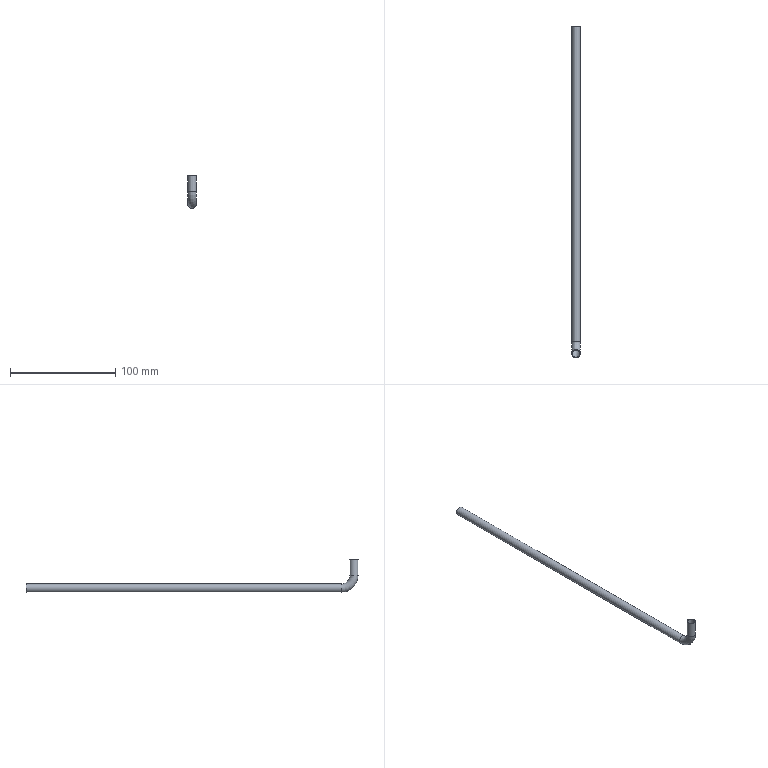Part | STEP file | 1-26.1 | 1 solid | 8 faces | box 8 x 315 x 31 mm | volume 5686 mm3 | cylinder 4 | torus 2 | plane 2 | commonest cylinder face diameters 6.5 x2 8 x2
STEP:
#1=CARTESIAN_POINT('',(0.,0.,0.));
#2=DIRECTION('',(0.,0.,1.));
#3=DIRECTION('',(1.,0.,0.));
#4=AXIS2_PLACEMENT_3D('',#1,#2,#3);
#5=CARTESIAN_POINT('',(-4.,311.,0.));
#6=VERTEX_POINT('',#5);
#7=CARTESIAN_POINT('',(0.,311.,0.));
#8=DIRECTION('',(0.,1.,0.));
#9=DIRECTION('',(-1.,0.,0.));
#10=AXIS2_PLACEMENT_3D('',#7,#8,#9);
#11=CIRCLE('',#10,4.);
#12=CARTESIAN_POINT('',(0.,311.,0.));
#13=DIRECTION('',(0.,-1.,0.));
#14=DIRECTION('',(-1.,0.,0.));
#15=AXIS2_PLACEMENT_3D('',#12,#13,#14);
#16=CYLINDRICAL_SURFACE('',#15,4.);
#17=CARTESIAN_POINT('',(6.283,0.));
#18=DIRECTION('',(-1.,0.));
#19=VECTOR('',#18,1.);
#20=LINE('',#17,#19);
#21=(GEOMETRIC_REPRESENTATION_CONTEXT(2)PARAMETRIC_REPRESENTATION_CONTEXT()REPRESENTATION_CONTEXT('',''));
#22=DEFINITIONAL_REPRESENTATION('',(#20),#21);
#23=PCURVE('',#16,#22);
#24=CARTESIAN_POINT('',(0.,311.,0.));
#25=DIRECTION('',(0.,1.,0.));
#26=DIRECTION('',(0.,0.,1.));
#27=AXIS2_PLACEMENT_3D('',#24,#25,#26);
#28=PLANE('',#27);
#29=CARTESIAN_POINT('',(0.,0.));
#30=DIRECTION('',(0.,-1.));
#31=AXIS2_PLACEMENT_2D('',#29,#30);
#32=CIRCLE('',#31,4.);
#33=(GEOMETRIC_REPRESENTATION_CONTEXT(2)PARAMETRIC_REPRESENTATION_CONTEXT()REPRESENTATION_CONTEXT('',''));
#34=DEFINITIONAL_REPRESENTATION('',(#32),#33);
#35=PCURVE('',#28,#34);
#36=SURFACE_CURVE('',#11,(#23,#35),.PCURVE_S1.);
#37=EDGE_CURVE('',#6,#6,#36,.T.);
#38=ORIENTED_EDGE('',*,*,#37,.F.);
#39=CARTESIAN_POINT('',(-4.,12.,0.));
#40=VERTEX_POINT('',#39);
#41=CARTESIAN_POINT('',(-4.,311.,0.));
#42=DIRECTION('',(0.,-1.,0.));
#43=VECTOR('',#42,1.);
#44=LINE('',#41,#43);
#45=CARTESIAN_POINT('',(6.283,0.));
#46=DIRECTION('',(0.,1.));
#47=VECTOR('',#46,1.);
#48=LINE('',#45,#47);
#49=(GEOMETRIC_REPRESENTATION_CONTEXT(2)PARAMETRIC_REPRESENTATION_CONTEXT()REPRESENTATION_CONTEXT('',''));
#50=DEFINITIONAL_REPRESENTATION('',(#48),#49);
#51=PCURVE('',#16,#50);
#52=CARTESIAN_POINT('',(0.,0.));
#53=DIRECTION('',(0.,1.));
#54=VECTOR('',#53,1.);
#55=LINE('',#52,#54);
#56=(GEOMETRIC_REPRESENTATION_CONTEXT(2)PARAMETRIC_REPRESENTATION_CONTEXT()REPRESENTATION_CONTEXT('',''));
#57=DEFINITIONAL_REPRESENTATION('',(#55),#56);
#58=PCURVE('',#16,#57);
#59=SEAM_CURVE('',#44,(#51,#58),.PCURVE_S1.);
#60=EDGE_CURVE('',#6,#40,#59,.T.);
#61=ORIENTED_EDGE('',*,*,#60,.T.);
#62=CARTESIAN_POINT('',(0.,12.,0.));
#63=DIRECTION('',(0.,-1.,0.));
#64=DIRECTION('',(-1.,0.,0.));
#65=AXIS2_PLACEMENT_3D('',#62,#63,#64);
#66=CIRCLE('',#65,4.);
#67=CARTESIAN_POINT('',(0.,299.));
#68=DIRECTION('',(1.,0.));
#69=VECTOR('',#68,1.);
#70=LINE('',#67,#69);
#71=(GEOMETRIC_REPRESENTATION_CONTEXT(2)PARAMETRIC_REPRESENTATION_CONTEXT()REPRESENTATION_CONTEXT('',''));
#72=DEFINITIONAL_REPRESENTATION('',(#70),#71);
#73=PCURVE('',#16,#72);
#74=CARTESIAN_POINT('',(0.,12.,12.));
#75=DIRECTION('',(1.,0.,0.));
#76=DIRECTION('',(0.,0.,-1.));
#77=AXIS2_PLACEMENT_3D('',#74,#75,#76);
#78=TOROIDAL_SURFACE('',#77,12.,4.);
#79=CARTESIAN_POINT('',(6.283,-1.571));
#80=DIRECTION('',(0.,1.));
#81=VECTOR('',#80,1.);
#82=LINE('',#79,#81);
#83=(GEOMETRIC_REPRESENTATION_CONTEXT(2)PARAMETRIC_REPRESENTATION_CONTEXT()REPRESENTATION_CONTEXT('',''));
#84=DEFINITIONAL_REPRESENTATION('',(#82),#83);
#85=PCURVE('',#78,#84);
#86=SURFACE_CURVE('',#66,(#73,#85),.PCURVE_S1.);
#87=EDGE_CURVE('',#40,#40,#86,.T.);
#88=ORIENTED_EDGE('',*,*,#87,.F.);
#89=ORIENTED_EDGE('',*,*,#60,.F.);
#90=EDGE_LOOP('',(#38,#61,#88,#89));
#91=FACE_BOUND('',#90,.T.);
#92=ADVANCED_FACE('',(#91),#16,.T.);
#93=ORIENTED_EDGE('',*,*,#87,.T.);
#94=CARTESIAN_POINT('',(-4.,0.,12.));
#95=VERTEX_POINT('',#94);
#96=CARTESIAN_POINT('',(-4.,12.,12.));
#97=DIRECTION('',(-1.,0.,0.));
#98=DIRECTION('',(0.,0.,-1.));
#99=AXIS2_PLACEMENT_3D('',#96,#97,#98);
#100=CIRCLE('',#99,12.);
#101=CARTESIAN_POINT('',(6.283,4.712));
#102=DIRECTION('',(-1.,0.));
#103=VECTOR('',#102,1.);
#104=LINE('',#101,#103);
#105=(GEOMETRIC_REPRESENTATION_CONTEXT(2)PARAMETRIC_REPRESENTATION_CONTEXT()REPRESENTATION_CONTEXT('',''));
#106=DEFINITIONAL_REPRESENTATION('',(#104),#105);
#107=PCURVE('',#78,#106);
#108=CARTESIAN_POINT('',(6.283,-1.571));
#109=DIRECTION('',(-1.,0.));
#110=VECTOR('',#109,1.);
#111=LINE('',#108,#110);
#112=(GEOMETRIC_REPRESENTATION_CONTEXT(2)PARAMETRIC_REPRESENTATION_CONTEXT()REPRESENTATION_CONTEXT('',''));
#113=DEFINITIONAL_REPRESENTATION('',(#111),#112);
#114=PCURVE('',#78,#113);
#115=SEAM_CURVE('',#100,(#107,#114),.PCURVE_S1.);
#116=EDGE_CURVE('',#40,#95,#115,.T.);
#117=ORIENTED_EDGE('',*,*,#116,.T.);
#118=CARTESIAN_POINT('',(4.,0.,12.));
#119=VERTEX_POINT('',#118);
#120=CARTESIAN_POINT('',(0.,0.,12.));
#121=DIRECTION('',(0.,0.,-1.));
#122=DIRECTION('',(-1.,0.,0.));
#123=AXIS2_PLACEMENT_3D('',#120,#121,#122);
#124=CIRCLE('',#123,4.);
#125=CARTESIAN_POINT('',(4.712,4.712));
#126=DIRECTION('',(0.,-1.));
#127=VECTOR('',#126,1.);
#128=LINE('',#125,#127);
#129=(GEOMETRIC_REPRESENTATION_CONTEXT(2)PARAMETRIC_REPRESENTATION_CONTEXT()REPRESENTATION_CONTEXT('',''));
#130=DEFINITIONAL_REPRESENTATION('',(#128),#129);
#131=PCURVE('',#78,#130);
#132=CARTESIAN_POINT('',(0.,0.,12.));
#133=DIRECTION('',(0.,0.,1.));
#134=DIRECTION('',(1.,0.,0.));
#135=AXIS2_PLACEMENT_3D('',#132,#133,#134);
#136=CYLINDRICAL_SURFACE('',#135,4.);
#137=CARTESIAN_POINT('',(3.142,0.));
#138=DIRECTION('',(-1.,0.));
#139=VECTOR('',#138,1.);
#140=LINE('',#137,#139);
#141=(GEOMETRIC_REPRESENTATION_CONTEXT(2)PARAMETRIC_REPRESENTATION_CONTEXT()REPRESENTATION_CONTEXT('',''));
#142=DEFINITIONAL_REPRESENTATION('',(#140),#141);
#143=PCURVE('',#136,#142);
#144=SURFACE_CURVE('',#124,(#131,#143),.PCURVE_S1.);
#145=EDGE_CURVE('',#95,#119,#144,.T.);
#146=ORIENTED_EDGE('',*,*,#145,.T.);
#147=CARTESIAN_POINT('',(0.,0.,12.));
#148=DIRECTION('',(0.,0.,-1.));
#149=DIRECTION('',(1.,0.,0.));
#150=AXIS2_PLACEMENT_3D('',#147,#148,#149);
#151=CIRCLE('',#150,4.);
#152=CARTESIAN_POINT('',(4.712,1.571));
#153=DIRECTION('',(0.,-1.));
#154=VECTOR('',#153,1.);
#155=LINE('',#152,#154);
#156=(GEOMETRIC_REPRESENTATION_CONTEXT(2)PARAMETRIC_REPRESENTATION_CONTEXT()REPRESENTATION_CONTEXT('',''));
#157=DEFINITIONAL_REPRESENTATION('',(#155),#156);
#158=PCURVE('',#78,#157);
#159=CARTESIAN_POINT('',(6.283,0.));
#160=DIRECTION('',(-1.,0.));
#161=VECTOR('',#160,1.);
#162=LINE('',#159,#161);
#163=(GEOMETRIC_REPRESENTATION_CONTEXT(2)PARAMETRIC_REPRESENTATION_CONTEXT()REPRESENTATION_CONTEXT('',''));
#164=DEFINITIONAL_REPRESENTATION('',(#162),#163);
#165=PCURVE('',#136,#164);
#166=SURFACE_CURVE('',#151,(#158,#165),.PCURVE_S1.);
#167=EDGE_CURVE('',#119,#95,#166,.T.);
#168=ORIENTED_EDGE('',*,*,#167,.T.);
#169=ORIENTED_EDGE('',*,*,#116,.F.);
#170=EDGE_LOOP('',(#93,#117,#146,#168,#169));
#171=FACE_BOUND('',#170,.T.);
#172=ADVANCED_FACE('',(#171),#78,.T.);
#173=ORIENTED_EDGE('',*,*,#145,.F.);
#174=ORIENTED_EDGE('',*,*,#167,.F.);
#175=CARTESIAN_POINT('',(4.,0.,27.));
#176=VERTEX_POINT('',#175);
#177=CARTESIAN_POINT('',(4.,0.,12.));
#178=DIRECTION('',(0.,0.,1.));
#179=VECTOR('',#178,1.);
#180=LINE('',#177,#179);
#181=CARTESIAN_POINT('',(6.283,0.));
#182=DIRECTION('',(0.,1.));
#183=VECTOR('',#182,1.);
#184=LINE('',#181,#183);
#185=(GEOMETRIC_REPRESENTATION_CONTEXT(2)PARAMETRIC_REPRESENTATION_CONTEXT()REPRESENTATION_CONTEXT('',''));
#186=DEFINITIONAL_REPRESENTATION('',(#184),#185);
#187=PCURVE('',#136,#186);
#188=CARTESIAN_POINT('',(0.,0.));
#189=DIRECTION('',(0.,1.));
#190=VECTOR('',#189,1.);
#191=LINE('',#188,#190);
#192=(GEOMETRIC_REPRESENTATION_CONTEXT(2)PARAMETRIC_REPRESENTATION_CONTEXT()REPRESENTATION_CONTEXT('',''));
#193=DEFINITIONAL_REPRESENTATION('',(#191),#192);
#194=PCURVE('',#136,#193);
#195=SEAM_CURVE('',#180,(#187,#194),.PCURVE_S1.);
#196=EDGE_CURVE('',#119,#176,#195,.T.);
#197=ORIENTED_EDGE('',*,*,#196,.T.);
#198=CARTESIAN_POINT('',(0.,0.,27.));
#199=DIRECTION('',(0.,0.,1.));
#200=DIRECTION('',(1.,0.,0.));
#201=AXIS2_PLACEMENT_3D('',#198,#199,#200);
#202=CIRCLE('',#201,4.);
#203=CARTESIAN_POINT('',(0.,15.));
#204=DIRECTION('',(1.,0.));
#205=VECTOR('',#204,1.);
#206=LINE('',#203,#205);
#207=(GEOMETRIC_REPRESENTATION_CONTEXT(2)PARAMETRIC_REPRESENTATION_CONTEXT()REPRESENTATION_CONTEXT('',''));
#208=DEFINITIONAL_REPRESENTATION('',(#206),#207);
#209=PCURVE('',#136,#208);
#210=CARTESIAN_POINT('',(0.,0.,27.));
#211=DIRECTION('',(0.,0.,1.));
#212=DIRECTION('',(1.,0.,0.));
#213=AXIS2_PLACEMENT_3D('',#210,#211,#212);
#214=PLANE('',#213);
#215=CARTESIAN_POINT('',(0.,0.));
#216=DIRECTION('',(1.,0.));
#217=AXIS2_PLACEMENT_2D('',#215,#216);
#218=CIRCLE('',#217,4.);
#219=(GEOMETRIC_REPRESENTATION_CONTEXT(2)PARAMETRIC_REPRESENTATION_CONTEXT()REPRESENTATION_CONTEXT('',''));
#220=DEFINITIONAL_REPRESENTATION('',(#218),#219);
#221=PCURVE('',#214,#220);
#222=SURFACE_CURVE('',#202,(#209,#221),.PCURVE_S1.);
#223=EDGE_CURVE('',#176,#176,#222,.T.);
#224=ORIENTED_EDGE('',*,*,#223,.F.);
#225=ORIENTED_EDGE('',*,*,#196,.F.);
#226=EDGE_LOOP('',(#173,#174,#197,#224,#225));
#227=FACE_BOUND('',#226,.T.);
#228=ADVANCED_FACE('',(#227),#136,.T.);
#229=ORIENTED_EDGE('',*,*,#37,.T.);
#230=EDGE_LOOP('',(#229));
#231=FACE_BOUND('',#230,.T.);
#232=CARTESIAN_POINT('',(-3.25,311.,0.));
#233=VERTEX_POINT('',#232);
#234=CARTESIAN_POINT('',(0.,311.,0.));
#235=DIRECTION('',(0.,1.,0.));
#236=DIRECTION('',(-1.,0.,0.));
#237=AXIS2_PLACEMENT_3D('',#234,#235,#236);
#238=CIRCLE('',#237,3.25);
#239=CARTESIAN_POINT('',(0.,0.));
#240=DIRECTION('',(0.,-1.));
#241=AXIS2_PLACEMENT_2D('',#239,#240);
#242=CIRCLE('',#241,3.25);
#243=(GEOMETRIC_REPRESENTATION_CONTEXT(2)PARAMETRIC_REPRESENTATION_CONTEXT()REPRESENTATION_CONTEXT('',''));
#244=DEFINITIONAL_REPRESENTATION('',(#242),#243);
#245=PCURVE('',#28,#244);
#246=CARTESIAN_POINT('',(0.,311.,0.));
#247=DIRECTION('',(0.,-1.,0.));
#248=DIRECTION('',(-1.,0.,0.));
#249=AXIS2_PLACEMENT_3D('',#246,#247,#248);
#250=CYLINDRICAL_SURFACE('',#249,3.25);
#251=CARTESIAN_POINT('',(6.283,0.));
#252=DIRECTION('',(-1.,0.));
#253=VECTOR('',#252,1.);
#254=LINE('',#251,#253);
#255=(GEOMETRIC_REPRESENTATION_CONTEXT(2)PARAMETRIC_REPRESENTATION_CONTEXT()REPRESENTATION_CONTEXT('',''));
#256=DEFINITIONAL_REPRESENTATION('',(#254),#255);
#257=PCURVE('',#250,#256);
#258=SURFACE_CURVE('',#238,(#245,#257),.PCURVE_S1.);
#259=EDGE_CURVE('',#233,#233,#258,.T.);
#260=ORIENTED_EDGE('',*,*,#259,.F.);
#261=EDGE_LOOP('',(#260));
#262=FACE_BOUND('',#261,.T.);
#263=ADVANCED_FACE('',(#231,#262),#28,.T.);
#264=ORIENTED_EDGE('',*,*,#223,.T.);
#265=EDGE_LOOP('',(#264));
#266=FACE_BOUND('',#265,.T.);
#267=CARTESIAN_POINT('',(3.25,0.,27.));
#268=VERTEX_POINT('',#267);
#269=CARTESIAN_POINT('',(0.,0.,27.));
#270=DIRECTION('',(0.,0.,1.));
#271=DIRECTION('',(1.,0.,0.));
#272=AXIS2_PLACEMENT_3D('',#269,#270,#271);
#273=CIRCLE('',#272,3.25);
#274=CARTESIAN_POINT('',(0.,0.));
#275=DIRECTION('',(1.,0.));
#276=AXIS2_PLACEMENT_2D('',#274,#275);
#277=CIRCLE('',#276,3.25);
#278=(GEOMETRIC_REPRESENTATION_CONTEXT(2)PARAMETRIC_REPRESENTATION_CONTEXT()REPRESENTATION_CONTEXT('',''));
#279=DEFINITIONAL_REPRESENTATION('',(#277),#278);
#280=PCURVE('',#214,#279);
#281=CARTESIAN_POINT('',(0.,0.,12.));
#282=DIRECTION('',(0.,0.,1.));
#283=DIRECTION('',(1.,0.,0.));
#284=AXIS2_PLACEMENT_3D('',#281,#282,#283);
#285=CYLINDRICAL_SURFACE('',#284,3.25);
#286=CARTESIAN_POINT('',(0.,15.));
#287=DIRECTION('',(1.,0.));
#288=VECTOR('',#287,1.);
#289=LINE('',#286,#288);
#290=(GEOMETRIC_REPRESENTATION_CONTEXT(2)PARAMETRIC_REPRESENTATION_CONTEXT()REPRESENTATION_CONTEXT('',''));
#291=DEFINITIONAL_REPRESENTATION('',(#289),#290);
#292=PCURVE('',#285,#291);
#293=SURFACE_CURVE('',#273,(#280,#292),.PCURVE_S1.);
#294=EDGE_CURVE('',#268,#268,#293,.T.);
#295=ORIENTED_EDGE('',*,*,#294,.F.);
#296=EDGE_LOOP('',(#295));
#297=FACE_BOUND('',#296,.T.);
#298=ADVANCED_FACE('',(#266,#297),#214,.T.);
#299=ORIENTED_EDGE('',*,*,#259,.F.);
#300=CARTESIAN_POINT('',(-3.25,12.,0.));
#301=VERTEX_POINT('',#300);
#302=CARTESIAN_POINT('',(-3.25,311.,0.));
#303=DIRECTION('',(0.,-1.,0.));
#304=VECTOR('',#303,1.);
#305=LINE('',#302,#304);
#306=CARTESIAN_POINT('',(6.283,0.));
#307=DIRECTION('',(0.,1.));
#308=VECTOR('',#307,1.);
#309=LINE('',#306,#308);
#310=(GEOMETRIC_REPRESENTATION_CONTEXT(2)PARAMETRIC_REPRESENTATION_CONTEXT()REPRESENTATION_CONTEXT('',''));
#311=DEFINITIONAL_REPRESENTATION('',(#309),#310);
#312=PCURVE('',#250,#311);
#313=CARTESIAN_POINT('',(0.,0.));
#314=DIRECTION('',(0.,1.));
#315=VECTOR('',#314,1.);
#316=LINE('',#313,#315);
#317=(GEOMETRIC_REPRESENTATION_CONTEXT(2)PARAMETRIC_REPRESENTATION_CONTEXT()REPRESENTATION_CONTEXT('',''));
#318=DEFINITIONAL_REPRESENTATION('',(#316),#317);
#319=PCURVE('',#250,#318);
#320=SEAM_CURVE('',#305,(#312,#319),.PCURVE_S1.);
#321=EDGE_CURVE('',#233,#301,#320,.T.);
#322=ORIENTED_EDGE('',*,*,#321,.T.);
#323=CARTESIAN_POINT('',(0.,12.,0.));
#324=DIRECTION('',(0.,-1.,0.));
#325=DIRECTION('',(-1.,0.,0.));
#326=AXIS2_PLACEMENT_3D('',#323,#324,#325);
#327=CIRCLE('',#326,3.25);
#328=CARTESIAN_POINT('',(0.,299.));
#329=DIRECTION('',(1.,0.));
#330=VECTOR('',#329,1.);
#331=LINE('',#328,#330);
#332=(GEOMETRIC_REPRESENTATION_CONTEXT(2)PARAMETRIC_REPRESENTATION_CONTEXT()REPRESENTATION_CONTEXT('',''));
#333=DEFINITIONAL_REPRESENTATION('',(#331),#332);
#334=PCURVE('',#250,#333);
#335=CARTESIAN_POINT('',(0.,12.,12.));
#336=DIRECTION('',(1.,0.,0.));
#337=DIRECTION('',(0.,0.,-1.));
#338=AXIS2_PLACEMENT_3D('',#335,#336,#337);
#339=TOROIDAL_SURFACE('',#338,12.,3.25);
#340=CARTESIAN_POINT('',(6.283,-1.571));
#341=DIRECTION('',(0.,1.));
#342=VECTOR('',#341,1.);
#343=LINE('',#340,#342);
#344=(GEOMETRIC_REPRESENTATION_CONTEXT(2)PARAMETRIC_REPRESENTATION_CONTEXT()REPRESENTATION_CONTEXT('',''));
#345=DEFINITIONAL_REPRESENTATION('',(#343),#344);
#346=PCURVE('',#339,#345);
#347=SURFACE_CURVE('',#327,(#334,#346),.PCURVE_S1.);
#348=EDGE_CURVE('',#301,#301,#347,.T.);
#349=ORIENTED_EDGE('',*,*,#348,.F.);
#350=ORIENTED_EDGE('',*,*,#321,.F.);
#351=EDGE_LOOP('',(#299,#322,#349,#350));
#352=FACE_BOUND('',#351,.F.);
#353=ADVANCED_FACE('',(#352),#250,.F.);
#354=ORIENTED_EDGE('',*,*,#348,.T.);
#355=CARTESIAN_POINT('',(-3.25,0.,12.));
#356=VERTEX_POINT('',#355);
#357=CARTESIAN_POINT('',(-3.25,12.,12.));
#358=DIRECTION('',(-1.,0.,0.));
#359=DIRECTION('',(0.,0.,-1.));
#360=AXIS2_PLACEMENT_3D('',#357,#358,#359);
#361=CIRCLE('',#360,12.);
#362=CARTESIAN_POINT('',(6.283,4.712));
#363=DIRECTION('',(-1.,0.));
#364=VECTOR('',#363,1.);
#365=LINE('',#362,#364);
#366=(GEOMETRIC_REPRESENTATION_CONTEXT(2)PARAMETRIC_REPRESENTATION_CONTEXT()REPRESENTATION_CONTEXT('',''));
#367=DEFINITIONAL_REPRESENTATION('',(#365),#366);
#368=PCURVE('',#339,#367);
#369=CARTESIAN_POINT('',(6.283,-1.571));
#370=DIRECTION('',(-1.,0.));
#371=VECTOR('',#370,1.);
#372=LINE('',#369,#371);
#373=(GEOMETRIC_REPRESENTATION_CONTEXT(2)PARAMETRIC_REPRESENTATION_CONTEXT()REPRESENTATION_CONTEXT('',''));
#374=DEFINITIONAL_REPRESENTATION('',(#372),#373);
#375=PCURVE('',#339,#374);
#376=SEAM_CURVE('',#361,(#368,#375),.PCURVE_S1.);
#377=EDGE_CURVE('',#301,#356,#376,.T.);
#378=ORIENTED_EDGE('',*,*,#377,.T.);
#379=CARTESIAN_POINT('',(3.25,0.,12.));
#380=VERTEX_POINT('',#379);
#381=CARTESIAN_POINT('',(0.,0.,12.));
#382=DIRECTION('',(0.,0.,-1.));
#383=DIRECTION('',(-1.,0.,0.));
#384=AXIS2_PLACEMENT_3D('',#381,#382,#383);
#385=CIRCLE('',#384,3.25);
#386=CARTESIAN_POINT('',(4.712,4.712));
#387=DIRECTION('',(0.,-1.));
#388=VECTOR('',#387,1.);
#389=LINE('',#386,#388);
#390=(GEOMETRIC_REPRESENTATION_CONTEXT(2)PARAMETRIC_REPRESENTATION_CONTEXT()REPRESENTATION_CONTEXT('',''));
#391=DEFINITIONAL_REPRESENTATION('',(#389),#390);
#392=PCURVE('',#339,#391);
#393=CARTESIAN_POINT('',(3.142,0.));
#394=DIRECTION('',(-1.,0.));
#395=VECTOR('',#394,1.);
#396=LINE('',#393,#395);
#397=(GEOMETRIC_REPRESENTATION_CONTEXT(2)PARAMETRIC_REPRESENTATION_CONTEXT()REPRESENTATION_CONTEXT('',''));
#398=DEFINITIONAL_REPRESENTATION('',(#396),#397);
#399=PCURVE('',#285,#398);
#400=SURFACE_CURVE('',#385,(#392,#399),.PCURVE_S1.);
#401=EDGE_CURVE('',#356,#380,#400,.T.);
#402=ORIENTED_EDGE('',*,*,#401,.T.);
#403=CARTESIAN_POINT('',(0.,0.,12.));
#404=DIRECTION('',(0.,0.,-1.));
#405=DIRECTION('',(1.,0.,0.));
#406=AXIS2_PLACEMENT_3D('',#403,#404,#405);
#407=CIRCLE('',#406,3.25);
#408=CARTESIAN_POINT('',(4.712,1.571));
#409=DIRECTION('',(0.,-1.));
#410=VECTOR('',#409,1.);
#411=LINE('',#408,#410);
#412=(GEOMETRIC_REPRESENTATION_CONTEXT(2)PARAMETRIC_REPRESENTATION_CONTEXT()REPRESENTATION_CONTEXT('',''));
#413=DEFINITIONAL_REPRESENTATION('',(#411),#412);
#414=PCURVE('',#339,#413);
#415=CARTESIAN_POINT('',(6.283,0.));
#416=DIRECTION('',(-1.,0.));
#417=VECTOR('',#416,1.);
#418=LINE('',#415,#417);
#419=(GEOMETRIC_REPRESENTATION_CONTEXT(2)PARAMETRIC_REPRESENTATION_CONTEXT()REPRESENTATION_CONTEXT('',''));
#420=DEFINITIONAL_REPRESENTATION('',(#418),#419);
#421=PCURVE('',#285,#420);
#422=SURFACE_CURVE('',#407,(#414,#421),.PCURVE_S1.);
#423=EDGE_CURVE('',#380,#356,#422,.T.);
#424=ORIENTED_EDGE('',*,*,#423,.T.);
#425=ORIENTED_EDGE('',*,*,#377,.F.);
#426=EDGE_LOOP('',(#354,#378,#402,#424,#425));
#427=FACE_BOUND('',#426,.F.);
#428=ADVANCED_FACE('',(#427),#339,.F.);
#429=ORIENTED_EDGE('',*,*,#401,.F.);
#430=ORIENTED_EDGE('',*,*,#423,.F.);
#431=CARTESIAN_POINT('',(3.25,0.,12.));
#432=DIRECTION('',(0.,0.,1.));
#433=VECTOR('',#432,1.);
#434=LINE('',#431,#433);
#435=CARTESIAN_POINT('',(6.283,0.));
#436=DIRECTION('',(0.,1.));
#437=VECTOR('',#436,1.);
#438=LINE('',#435,#437);
#439=(GEOMETRIC_REPRESENTATION_CONTEXT(2)PARAMETRIC_REPRESENTATION_CONTEXT()REPRESENTATION_CONTEXT('',''));
#440=DEFINITIONAL_REPRESENTATION('',(#438),#439);
#441=PCURVE('',#285,#440);
#442=CARTESIAN_POINT('',(0.,0.));
#443=DIRECTION('',(0.,1.));
#444=VECTOR('',#443,1.);
#445=LINE('',#442,#444);
#446=(GEOMETRIC_REPRESENTATION_CONTEXT(2)PARAMETRIC_REPRESENTATION_CONTEXT()REPRESENTATION_CONTEXT('',''));
#447=DEFINITIONAL_REPRESENTATION('',(#445),#446);
#448=PCURVE('',#285,#447);
#449=SEAM_CURVE('',#434,(#441,#448),.PCURVE_S1.);
#450=EDGE_CURVE('',#380,#268,#449,.T.);
#451=ORIENTED_EDGE('',*,*,#450,.T.);
#452=ORIENTED_EDGE('',*,*,#294,.F.);
#453=ORIENTED_EDGE('',*,*,#450,.F.);
#454=EDGE_LOOP('',(#429,#430,#451,#452,#453));
#455=FACE_BOUND('',#454,.F.);
#456=ADVANCED_FACE('',(#455),#285,.F.);
#457=CLOSED_SHELL('',(#92,#172,#228,#263,#298,#353,#428,#456));
#458=MANIFOLD_SOLID_BREP('',#457);
#459=(LENGTH_UNIT()NAMED_UNIT(*)SI_UNIT(.MILLI.,.METRE.));
#460=UNCERTAINTY_MEASURE_WITH_UNIT(LENGTH_MEASURE(0.0000001),#459,'','');
#461=(NAMED_UNIT(*)PLANE_ANGLE_UNIT()SI_UNIT($,.RADIAN.));
#462=(NAMED_UNIT(*)SI_UNIT($,.STERADIAN.)SOLID_ANGLE_UNIT());
#463=(GEOMETRIC_REPRESENTATION_CONTEXT(3)GLOBAL_UNCERTAINTY_ASSIGNED_CONTEXT((#460))GLOBAL_UNIT_ASSIGNED_CONTEXT((#459,#461,#462))REPRESENTATION_CONTEXT('',''));
#464=ADVANCED_BREP_SHAPE_REPRESENTATION('',(#4,#458),#463);